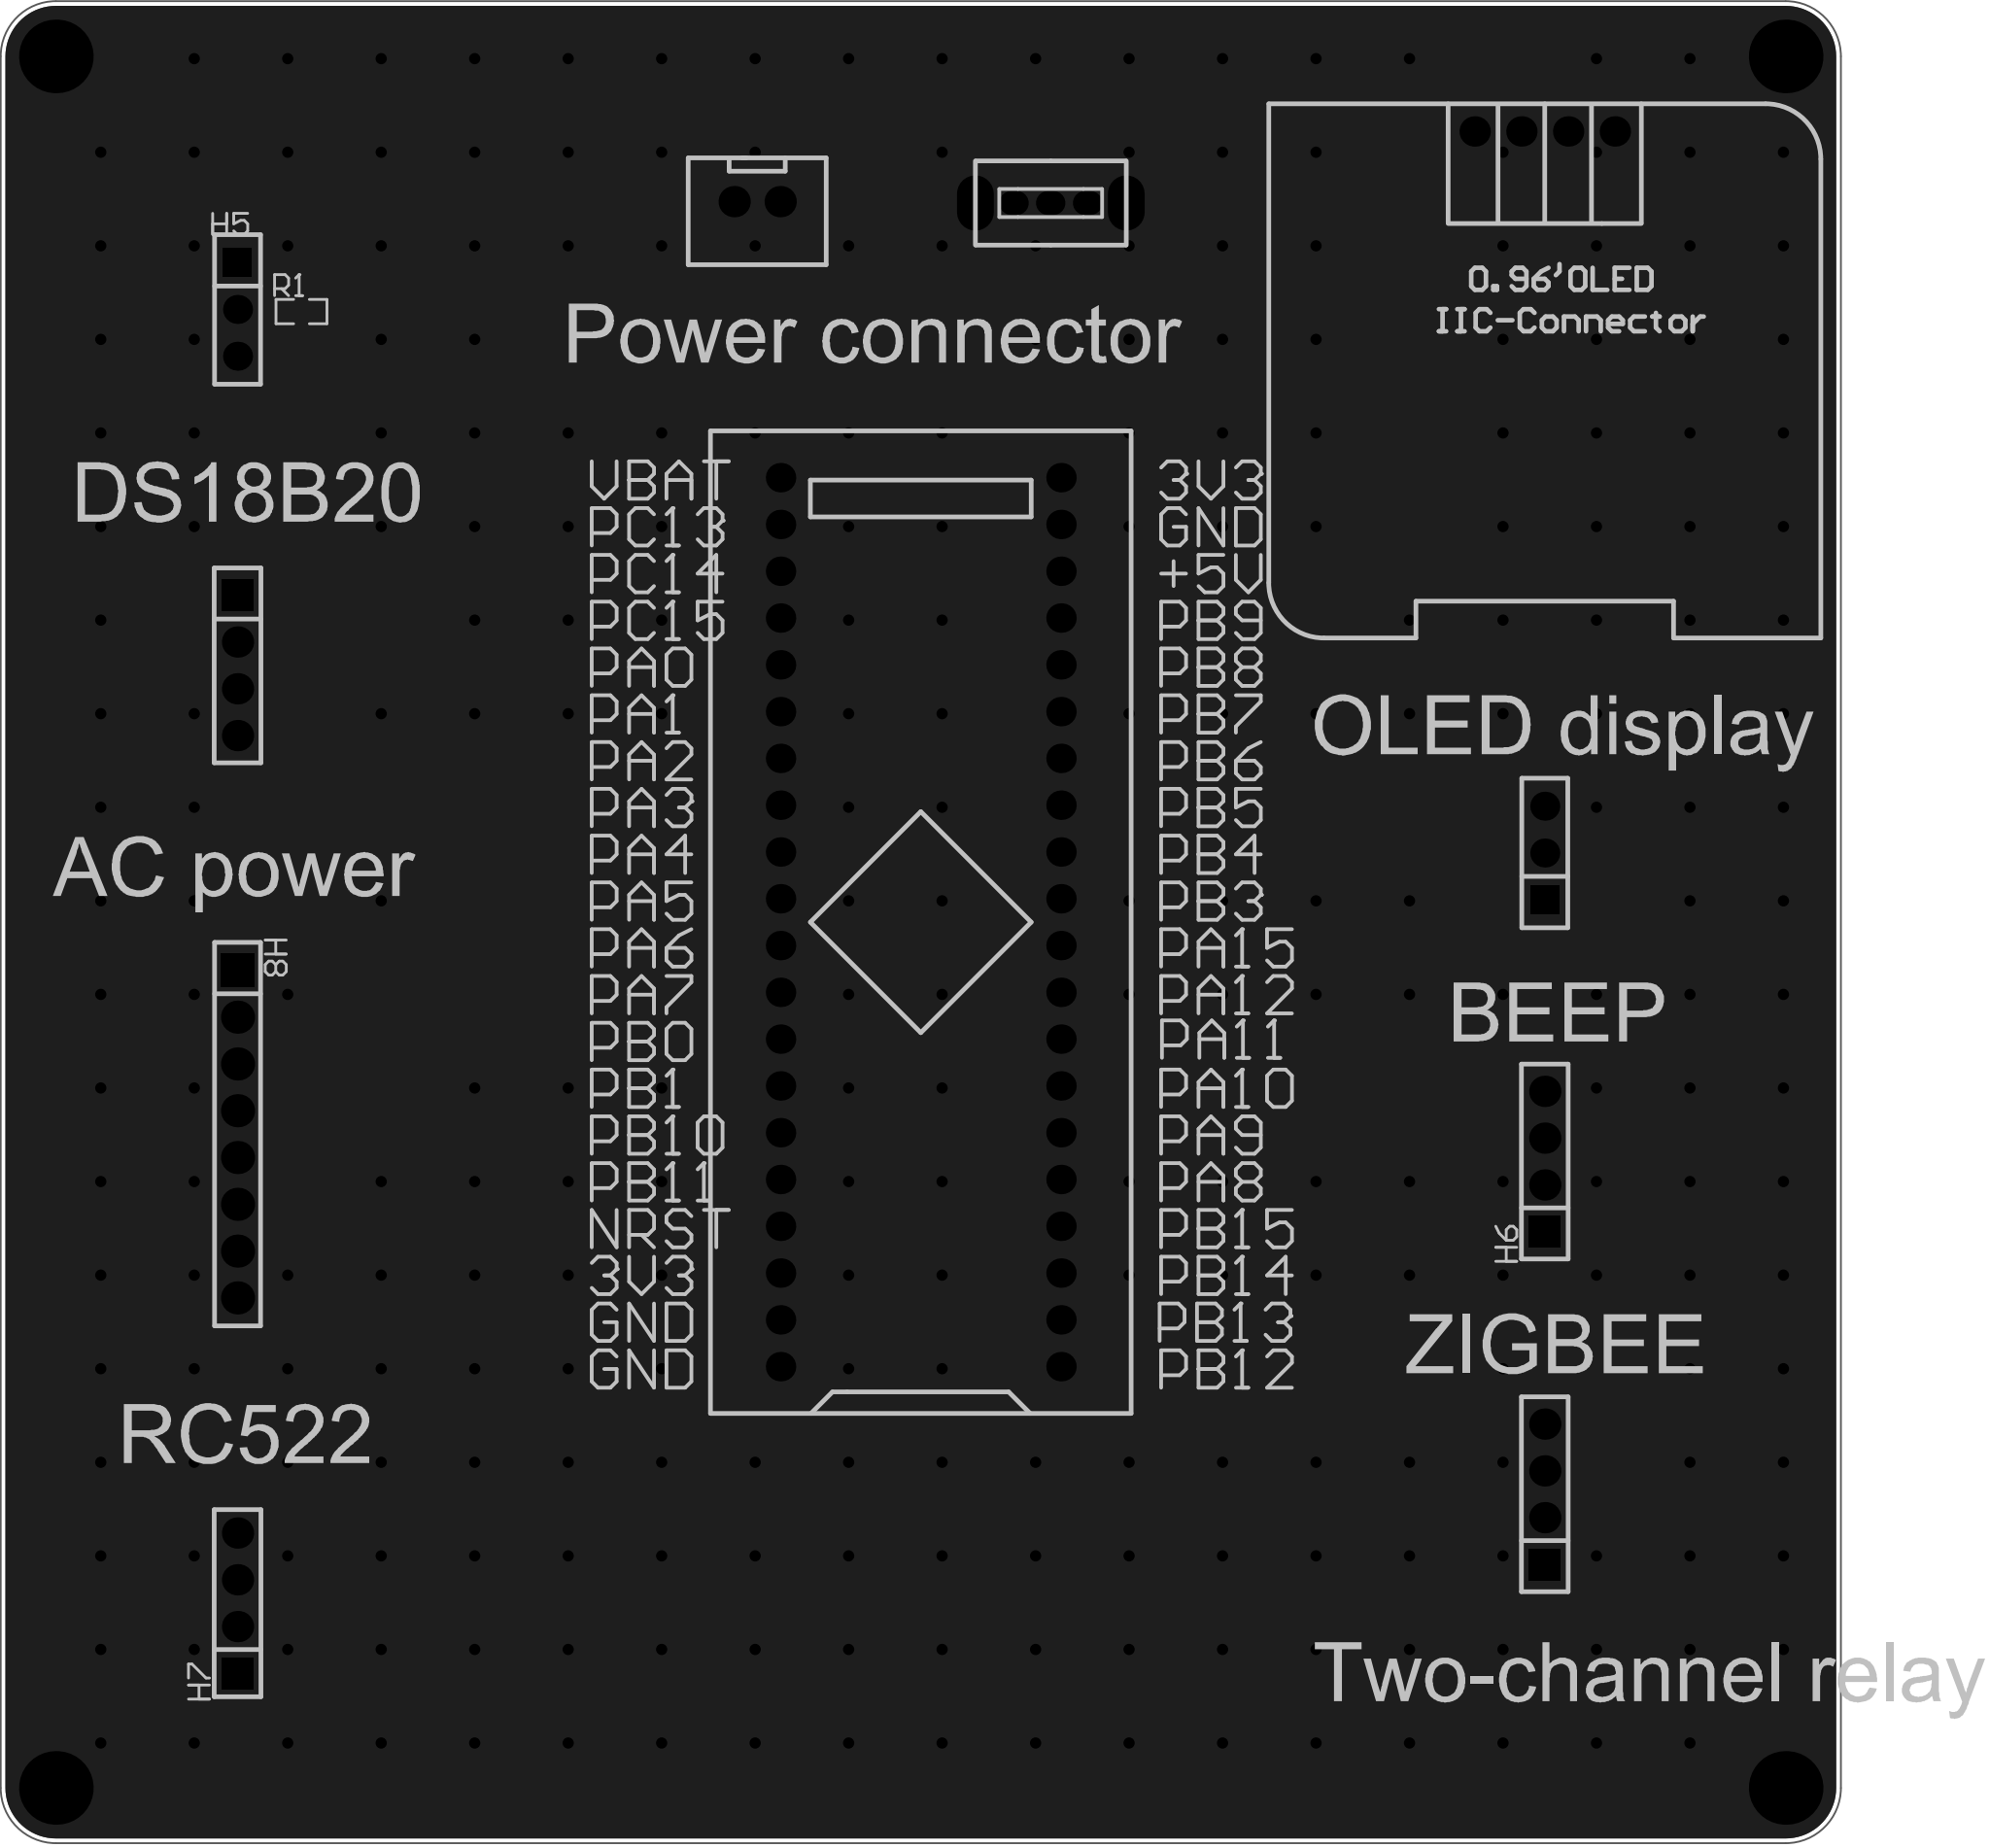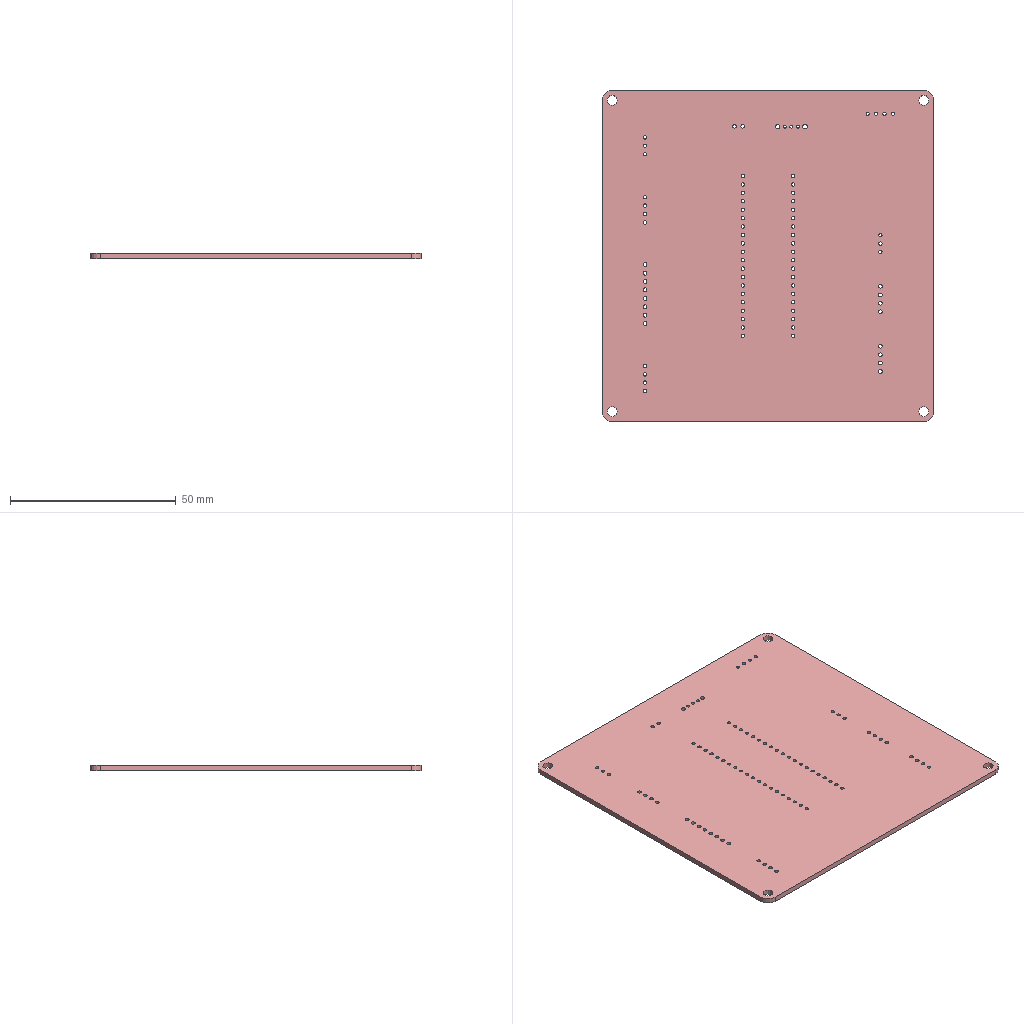Circuit board layout | Altium Designer | box 100 x 100 x 1.6 mm
Layer stack:
# Altium Designer layer stack of  (unit mm; dielectric type: 0 none, 1 core, 2 prepreg, 3 surface material)
index,name,kind,layer,copper_thickness_mm,dielectric_type,dielectric_thickness_mm,dielectric_material,dielectric_constant
0,Top Paste Mask Layer,other,,,,,,
1,Top Silkscreen Layer,other,,,,,,
2,Top Solder Mask Layer,dielectric,,,3,0.01,,3.3
3,Top Layer,copper,Top Layer,0.035,,,,
4,Dielectric1,dielectric,,,3,1.51,FR4,4.5
5,Bottom Layer,copper,Bottom Layer,0.035,,,,
6,Bottom Solder Mask Layer,dielectric,,,3,0.01,,3.3
7,Bottom Silkscreen Layer,other,,,,,,
8,Bottom Paste Mask Layer,other,,,,,,
# drill layer pairs: low layer,high layer
drill_pair,Top Layer,Bottom Layer
Part placement:
Designator,Comment,Layer,Footprint,Center-X(mm),Center-Y(mm),Rotation
U1,STM32F103C8T6-Card,TopLayer,CONN-TH_L53.3-W22.9_STM32F103C8T6-CARD,141.351,130.937,90
OLED1,,TopLayer,0.96OLED_4P,175.26,173.863,0
CN4,XH2.54*2P_through-hole,TopLayer,CONN-TH_2P-P2.50-XH2.54-2P,132.461,170.053,0
SW5,,TopLayer,拨动开关,148.417,169.978,0
H1,,TopLayer,HDR-TH_3P-P2.54-V-F,175.26,134.692,90
H2,,TopLayer,HDR-TH_4P-P2.54-V-F,104.223,144.876,270
H4,,TopLayer,HDR-TH_4P-P2.54-V-F,175.26,99.878,90
H5,,TopLayer,HDR-TH_3P-P2.54-V-F,104.223,164.2,270
H6,,TopLayer,HDR-TH_4P-P2.54-V-F,175.26,117.942,90
H7,,TopLayer,HDR-TH_4P-P2.54-V-M,104.223,93.966,90
H8,,TopLayer,HDR-TH_8P-P2.54-V-F-1,104.223,119.43,270
R1,4.7K,TopLayer,R0603,107.696,164.084,0
Pad and via stacks:
# Altium Designer via and pad stacks of  (unit mm). Each distinct definition once, with the count of objects using it.
# via: kind,start_layer,end_layer,hole_mm,diameter_mm,mode(0 simple;1 top-mid-bottom;2 full stack),diameter_per_layer,count,example_net
# pad: kind,layer,hole_mm,hole_type(0 round;1 square;2 slot),plating,top_size,top_shape(1 round;2 rect;3 octagon;9 rounded rect),mid_size,bottom_size,mode,footprint,size_per_layer,count,example
pad,Multi-Layer,3,0,plated,4x4,1,4x4,4x4,0,,,4,1
pad,Multi-Layer,1,0,plated,1.6x1.6,1,1.6x1.6,1.6x1.6,0,CONN-TH_L53.3-W22.9_STM32F103C8T6-CARD,,40,U1.1
pad,Multi-Layer,1,0,plated,1.65x1.65,1,1.65x1.65,1.65x1.65,0,0.96OLED_4P,,4,OLED1.4
pad,Multi-Layer,1.05,0,plated,1.7x1.7,1,1.7x1.7,1.7x1.7,0,CONN-TH_2P-P2.50-XH2.54-2P,,2,CN4.2
pad,Multi-Layer,0.8992,0,plated,1.6x1.3,1,1.6x1.3,1.6x1.3,0,\u00B2\u00A6\u00B6\u00AF\u00BF\u00AA\u00B9\u00D8,,3,SW5.1
pad,Multi-Layer,1.3,0,plated,3x1.999,1,3x1.999,3x1.999,0,\u00B2\u00A6\u00B6\u00AF\u00BF\u00AA\u00B9\u00D8,,2,SW5.4
pad,Multi-Layer,1.02,0,plated,1.575x1.575,1,1.575x1.575,1.575x1.575,0,HDR-TH_3P-P2.54-V-F,,4,H1.3
pad,Multi-Layer,1.02,0,plated,1.575x1.575,2,1.575x1.575,1.575x1.575,0,HDR-TH_3P-P2.54-V-F,,2,H1.1
pad,Multi-Layer,1.1,0,plated,1.7x1.7,2,1.7x1.7,1.7x1.7,0,HDR-TH_4P-P2.54-V-F,,3,H2.1
pad,Multi-Layer,1.1,0,plated,1.7x1.7,1,1.7x1.7,1.7x1.7,0,HDR-TH_4P-P2.54-V-F,,9,H2.2
pad,Multi-Layer,1.1,0,plated,1.7x1.7,2,1.7x1.7,1.7x1.7,0,HDR-TH_4P-P2.54-V-M,,1,H7.1
pad,Multi-Layer,1.1,0,plated,1.7x1.7,1,1.7x1.7,1.7x1.7,0,HDR-TH_4P-P2.54-V-M,,3,H7.2
pad,Multi-Layer,1.2,0,plated,1.8x1.8,2,1.8x1.8,1.8x1.8,0,HDR-TH_8P-P2.54-V-F-1,,1,H8.1
pad,Multi-Layer,1.2,0,plated,1.8x1.8,1,1.8x1.8,1.8x1.8,0,HDR-TH_8P-P2.54-V-F-1,,7,H8.2
pad,Top Layer,0,0,plated,0.8065x0.864,2,0.8065x0.864,0.8065x0.864,0,R0603,,2,R1.2
via,Top Layer,Bottom Layer,0.3048,0.61,0,,280,GND
Copper pours:
name,layer,net,type(0 solid;1 hatched;2 none)
Bottom Layer-GND,Bottom Layer,GND,0
Top Layer-GND,Top Layer,GND,0
Design rules, without the lines most boards share:
# Altium Designer design rules of  (exported by Altium Designer, unit mm)
# columns: name | kind | enabled | priority | scope1 | scope2 | descriptor | typed fields (field=value)
Copper_copperRegion_copperThickness1oz | 0 | disabled | 4 | All | All | Clearance Constraint (Gap=5.984mil) (Disabled)(All),(All) | gap=0.152
Copper_copperRegion_copperThickness1oz_1 | 63 | disabled | 4 | All | All | Board Clearance Constraint (Gap=0mil) (Disabled)(All) |
Copper_copperRegion_Copper_copperRegion | 0 | disabled | 5 | All | All | Clearance Constraint (Gap=5.984mil) (Disabled)(All),(All) | gap=0.152
Copper_copperRegion_Copper_copperRegion_1 | 63 | disabled | 5 | All | All | Board Clearance Constraint (Gap=0mil) (Disabled)(All) |
copperThickness1oz | 0 | enabled | 6 | All | All | Clearance Constraint (Gap=5.984mil) (All),(All) | gap=0.152
copperThickness1oz_1 | 63 | enabled | 6 | All | All | Board Clearance Constraint (Gap=0mil) (All) |
copperRegion_copperThickness1oz | 20 | disabled | 1 | All | All | Polygon Connect Rule(Relief Connect )(Conductor Width=10mil) (Relief Angle=90 Angle) (Entries=4) (Air Gap Width=10mil) (Disabled)(All),(All) | connect_style(0=relief,1=direct,2=none)=0 relief_conductor_width=0.254 relief_entries=4
copperRegion_Copper_copperRegion | 20 | disabled | 2 | All | All | Polygon Connect Rule(Relief Connect )(Conductor Width=10mil) (Relief Angle=90 Angle) (Entries=4) (Air Gap Width=10mil) (Disabled)(All),(All) | connect_style(0=relief,1=direct,2=none)=0 relief_conductor_width=0.254 relief_entries=4
copperRegion | 20 | enabled | 3 | All | All | Polygon Connect Rule(Relief Connect )(Conductor Width=10mil) (Relief Angle=90 Angle) (Entries=4) (Air Gap Width=10mil) (All),(All) | connect_style(0=relief,1=direct,2=none)=0 relief_conductor_width=0.254 relief_entries=4